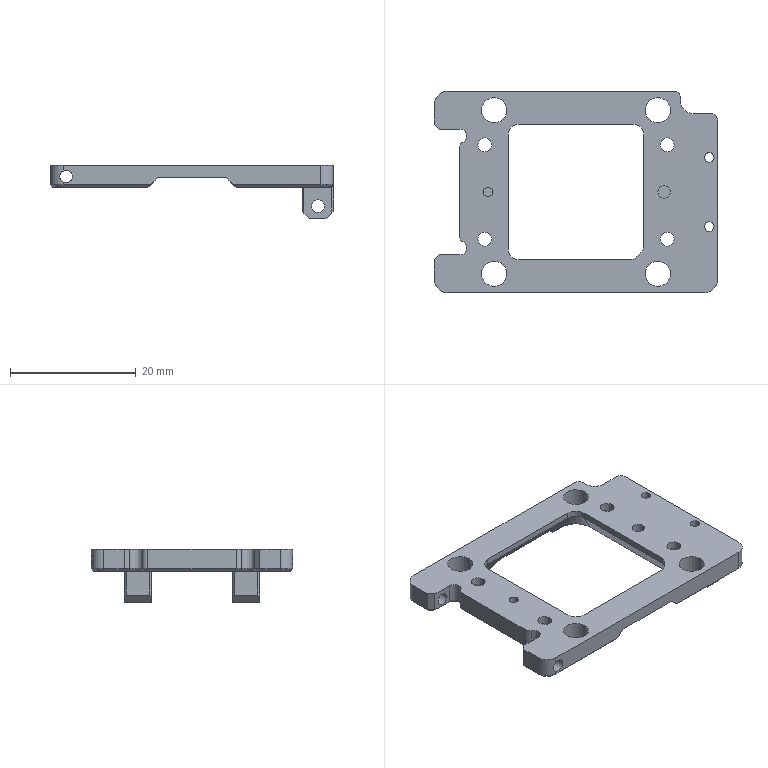Part | 2 solids | 382 faces | box 45 x 32 x 8.5 mm | volume 5048 mm3 | plane 214 | cylinder 114 | cone 34 | spline 20 | commonest cylinder face diameters 4 x40 2.2 x20 2.02 x16 3.6 x10 1.5 x8 2 x8